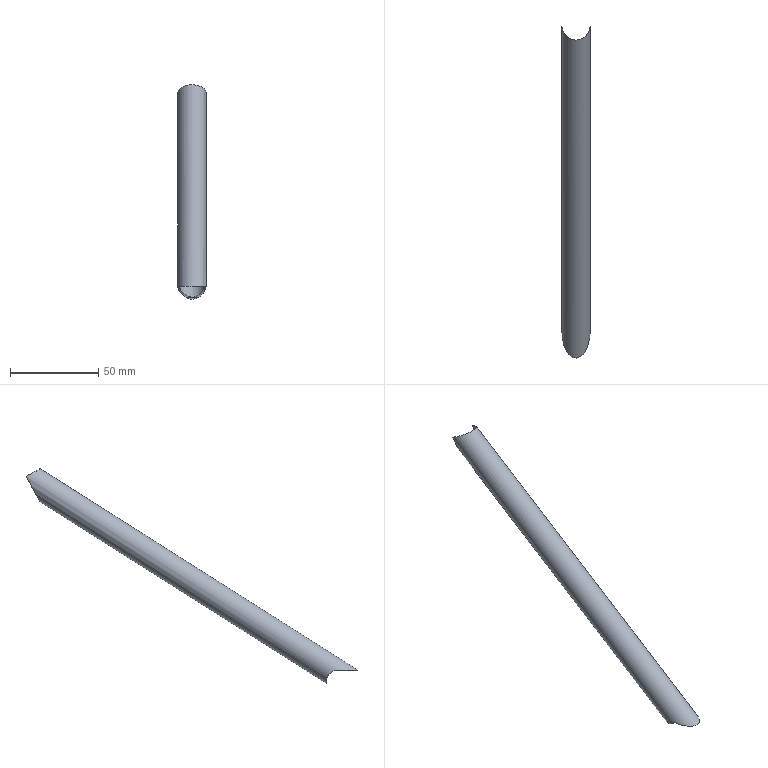Part | NX | features MG0313 aframe 2 | 1 solid | 6 faces | box 15.877 x 187.726 x 121.401 mm | volume 9582 mm3 | cylinder 4 | plane 2 | commonest cylinder face diameters 15.875 x2 13.31 x1 13.843 x1